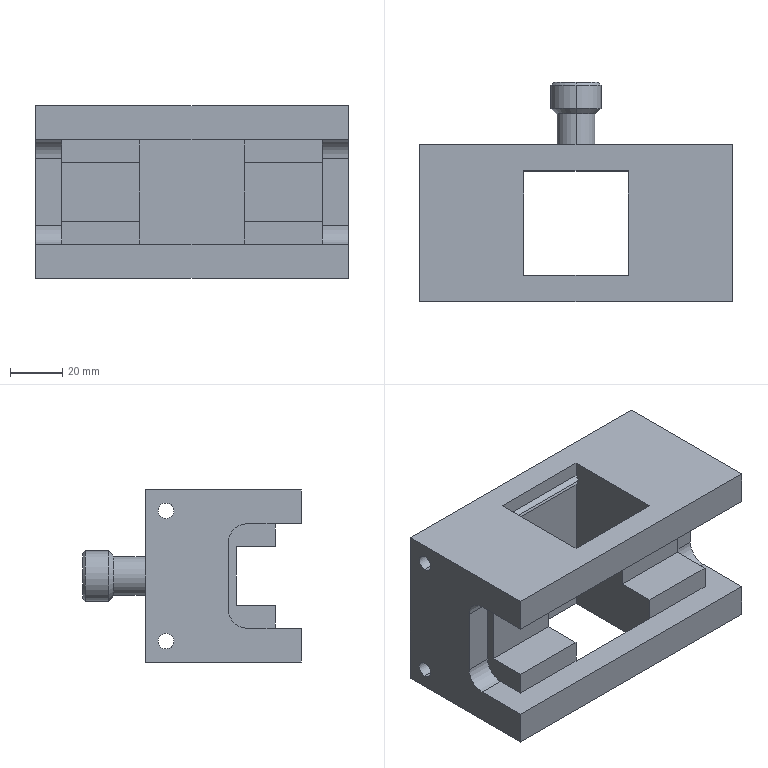Part | SolidWorks | features ICE 12, Chamfer 2, Fillet 2, Extrusion 1 | 1 solid | 78 faces | box 120 x 84 x 66 mm | volume 274299 mm3 | plane 44 | cylinder 30 | cone 4 | commonest cylinder face diameters 6 x12 14 x4 19.336 x4 20 x4 14.621 x2 24.815 x2